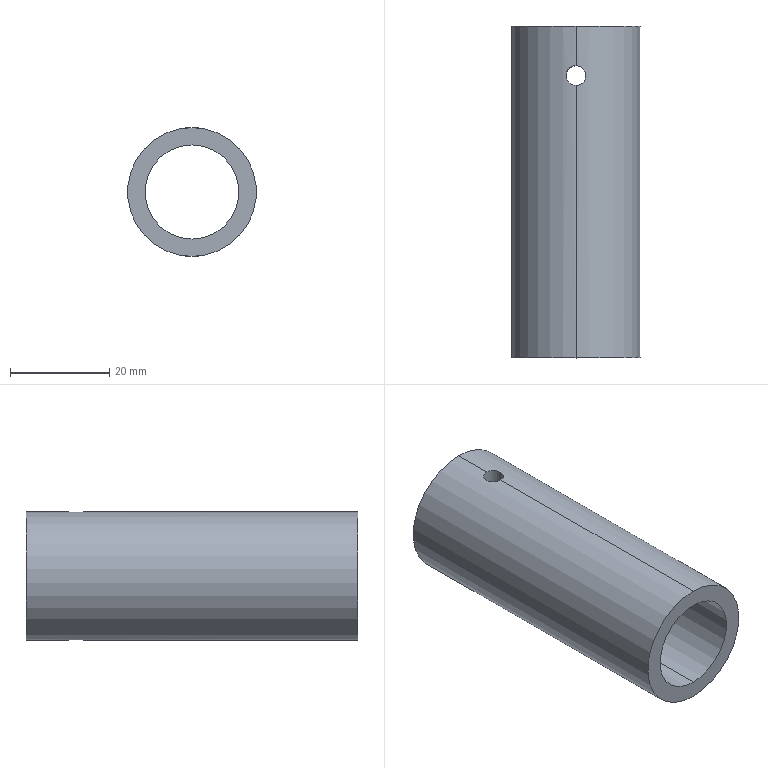Part | STEP file | PN_0064 | 1 solid | 10 faces | box 26 x 67 x 26 mm | volume 16488 mm3 | cylinder 8 | plane 2 | commonest cylinder face diameters 4 x4 19 x2 26 x2